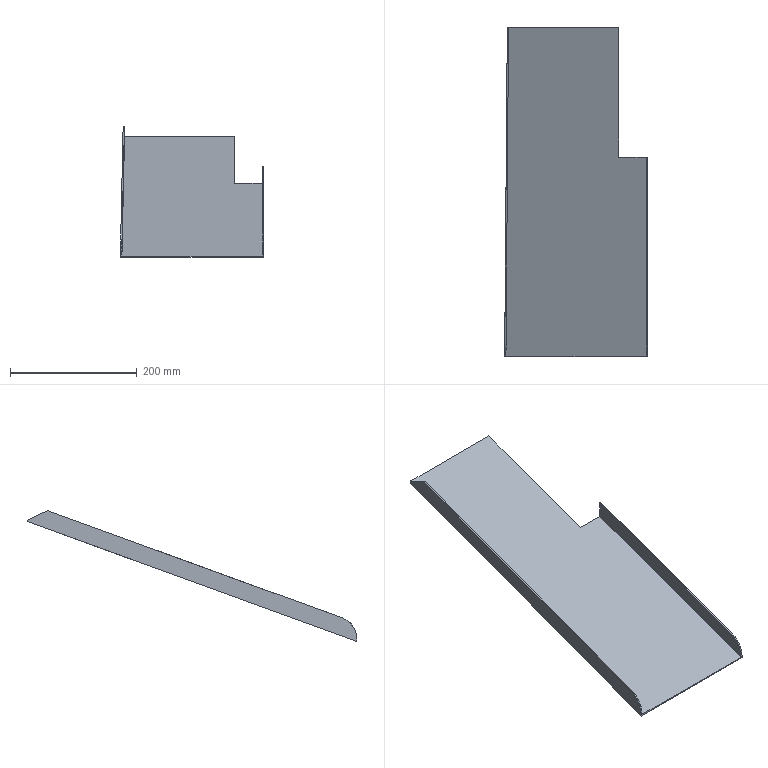Part | NX | features solid 2 | 1 solid | 15 faces | box 225.247 x 520 x 206.353 mm | volume 267602 mm3 | plane 9 | spline 5 | cylinder 1 | commonest cylinder face diameters 70 x1
STEP:
#1=CARTESIAN_POINT('',(-877.991,-100.,-231.58));
#2=VERTEX_POINT('',#1);
#3=CARTESIAN_POINT('',(-882.15,-620.,-420.844));
#4=VERTEX_POINT('',#3);
#5=CARTESIAN_POINT('',(-877.991,-100.,-231.58));
#6=CARTESIAN_POINT('',(-878.46,-143.332,-247.351));
#7=CARTESIAN_POINT('',(-879.198,-229.999,-278.895));
#8=CARTESIAN_POINT('',(-880.069,-338.332,-318.325));
#9=CARTESIAN_POINT('',(-880.798,-424.998,-349.869));
#10=CARTESIAN_POINT('',(-881.335,-511.666,-381.414));
#11=CARTESIAN_POINT('',(-881.837,-576.666,-405.072));
#12=CARTESIAN_POINT('',(-882.15,-620.,-420.844));
#13=B_SPLINE_CURVE_WITH_KNOTS('',3,(#5,#6,#7,#8,#9,#10,#11,#12),.UNSPECIFIED.,.F.,.F.,(4,1,1,1,1,4),(0.8331,0.9714,1.11,1.179,1.248,1.386),.UNSPECIFIED.);
#14=EDGE_CURVE('',#2,#4,#13,.T.);
#15=ORIENTED_EDGE('',*,*,#14,.T.);
#16=CARTESIAN_POINT('',(-660.908,-620.,-420.844));
#17=VERTEX_POINT('',#16);
#18=CARTESIAN_POINT('',(-1178.908,-620.,-420.844));
#19=DIRECTION('',(1.,0.,0.));
#20=VECTOR('',#19,1000.);
#21=LINE('',#18,#20);
#22=EDGE_CURVE('',#4,#17,#21,.T.);
#23=ORIENTED_EDGE('',*,*,#22,.T.);
#24=CARTESIAN_POINT('',(-660.908,-305.,-306.193));
#25=VERTEX_POINT('',#24);
#26=CARTESIAN_POINT('',(-660.908,-100.,-231.58));
#27=DIRECTION('',(0.,-0.9397,-0.342));
#28=VECTOR('',#27,1000.);
#29=LINE('',#26,#28);
#30=EDGE_CURVE('',#25,#17,#29,.T.);
#31=ORIENTED_EDGE('',*,*,#30,.F.);
#32=CARTESIAN_POINT('',(-703.908,-305.,-306.193));
#33=VERTEX_POINT('',#32);
#34=CARTESIAN_POINT('',(-1178.908,-305.,-306.193));
#35=DIRECTION('',(1.,0.,0.));
#36=VECTOR('',#35,1000.);
#37=LINE('',#34,#36);
#38=EDGE_CURVE('',#33,#25,#37,.T.);
#39=ORIENTED_EDGE('',*,*,#38,.F.);
#40=CARTESIAN_POINT('',(-703.908,-100.,-231.58));
#41=VERTEX_POINT('',#40);
#42=CARTESIAN_POINT('',(-703.908,-63.022,-218.121));
#43=DIRECTION('',(0.,-0.9397,-0.342));
#44=VECTOR('',#43,1000.);
#45=LINE('',#42,#44);
#46=EDGE_CURVE('',#41,#33,#45,.T.);
#47=ORIENTED_EDGE('',*,*,#46,.F.);
#48=CARTESIAN_POINT('',(-1178.908,-100.,-231.58));
#49=DIRECTION('',(1.,0.,0.));
#50=VECTOR('',#49,1000.);
#51=LINE('',#48,#50);
#52=EDGE_CURVE('',#2,#41,#51,.T.);
#53=ORIENTED_EDGE('',*,*,#52,.F.);
#54=EDGE_LOOP('',(#15,#23,#31,#39,#47,#53));
#55=FACE_BOUND('',#54,.T.);
#56=CARTESIAN_POINT('',(-1178.908,-63.022,-218.121));
#57=DIRECTION('',(0.,0.342,-0.9397));
#58=DIRECTION('',(-1.,0.,0.));
#59=AXIS2_PLACEMENT_3D('',#56,#57,#58);
#60=PLANE('',#59);
#61=ADVANCED_FACE('',(#55),#60,.F.);
#62=CARTESIAN_POINT('',(-879.998,-100.,-233.708));
#63=VERTEX_POINT('',#62);
#64=CARTESIAN_POINT('',(-703.908,-100.,-233.708));
#65=VERTEX_POINT('',#64);
#66=CARTESIAN_POINT('',(-1178.908,-100.,-233.708));
#67=DIRECTION('',(1.,0.,0.));
#68=VECTOR('',#67,1000.);
#69=LINE('',#66,#68);
#70=EDGE_CURVE('',#63,#65,#69,.T.);
#71=ORIENTED_EDGE('',*,*,#70,.T.);
#72=CARTESIAN_POINT('',(-703.908,-305.,-308.322));
#73=VERTEX_POINT('',#72);
#74=CARTESIAN_POINT('',(-703.908,-62.338,-220.));
#75=DIRECTION('',(0.,-0.9397,-0.342));
#76=VECTOR('',#75,1000.);
#77=LINE('',#74,#76);
#78=EDGE_CURVE('',#65,#73,#77,.T.);
#79=ORIENTED_EDGE('',*,*,#78,.T.);
#80=CARTESIAN_POINT('',(-658.908,-305.,-308.322));
#81=VERTEX_POINT('',#80);
#82=CARTESIAN_POINT('',(-1178.908,-305.,-308.322));
#83=DIRECTION('',(1.,0.,0.));
#84=VECTOR('',#83,1000.);
#85=LINE('',#82,#84);
#86=EDGE_CURVE('',#73,#81,#85,.T.);
#87=ORIENTED_EDGE('',*,*,#86,.T.);
#88=CARTESIAN_POINT('',(-658.908,-620.,-422.972));
#89=VERTEX_POINT('',#88);
#90=CARTESIAN_POINT('',(-658.908,-62.338,-220.));
#91=DIRECTION('',(0.,-0.9397,-0.342));
#92=VECTOR('',#91,1000.);
#93=LINE('',#90,#92);
#94=EDGE_CURVE('',#81,#89,#93,.T.);
#95=ORIENTED_EDGE('',*,*,#94,.T.);
#96=CARTESIAN_POINT('',(-884.155,-620.,-422.972));
#97=VERTEX_POINT('',#96);
#98=CARTESIAN_POINT('',(-1178.908,-620.,-422.972));
#99=DIRECTION('',(1.,0.,0.));
#100=VECTOR('',#99,1000.);
#101=LINE('',#98,#100);
#102=EDGE_CURVE('',#97,#89,#101,.T.);
#103=ORIENTED_EDGE('',*,*,#102,.F.);
#104=CARTESIAN_POINT('',(-879.998,-100.,-233.708));
#105=CARTESIAN_POINT('',(-880.468,-143.332,-249.48));
#106=CARTESIAN_POINT('',(-881.204,-229.999,-281.024));
#107=CARTESIAN_POINT('',(-882.073,-338.332,-320.454));
#108=CARTESIAN_POINT('',(-882.805,-424.999,-351.998));
#109=CARTESIAN_POINT('',(-883.339,-511.666,-383.542));
#110=CARTESIAN_POINT('',(-883.842,-576.666,-407.2));
#111=CARTESIAN_POINT('',(-884.155,-620.,-422.972));
#112=B_SPLINE_CURVE_WITH_KNOTS('',3,(#104,#105,#106,#107,#108,#109,#110,#111),.UNSPECIFIED.,.F.,.F.,(4,1,1,1,1,4),(2.341,2.479,2.617,2.687,2.756,2.894),.UNSPECIFIED.);
#113=EDGE_CURVE('',#63,#97,#112,.T.);
#114=ORIENTED_EDGE('',*,*,#113,.F.);
#115=EDGE_LOOP('',(#71,#79,#87,#95,#103,#114));
#116=FACE_BOUND('',#115,.T.);
#117=CARTESIAN_POINT('',(-1178.908,-62.338,-220.));
#118=DIRECTION('',(0.,0.342,-0.9397));
#119=DIRECTION('',(-1.,0.,0.));
#120=AXIS2_PLACEMENT_3D('',#117,#118,#119);
#121=PLANE('',#120);
#122=ADVANCED_FACE('',(#116),#121,.T.);
#123=CARTESIAN_POINT('',(-877.991,-100.,-231.556));
#124=VERTEX_POINT('',#123);
#125=CARTESIAN_POINT('',(-878.237,-132.013,-216.627));
#126=VERTEX_POINT('',#125);
#127=CARTESIAN_POINT('',(-877.991,-100.,-231.556));
#128=CARTESIAN_POINT('',(-878.076,-110.671,-226.579));
#129=CARTESIAN_POINT('',(-878.158,-121.342,-221.603));
#130=CARTESIAN_POINT('',(-878.237,-132.013,-216.627));
#131=B_SPLINE_CURVE_WITH_KNOTS('',3,(#127,#128,#129,#130),.UNSPECIFIED.,.F.,.F.,(4,4),(0.00003167,0.03536),.UNSPECIFIED.);
#132=EDGE_CURVE('',#124,#126,#131,.T.);
#133=ORIENTED_EDGE('',*,*,#132,.F.);
#134=CARTESIAN_POINT('',(-879.991,-100.,-231.54));
#135=VERTEX_POINT('',#134);
#136=CARTESIAN_POINT('',(-877.991,-100.,-231.556));
#137=CARTESIAN_POINT('',(-878.658,-100.,-231.55));
#138=CARTESIAN_POINT('',(-879.324,-100.,-231.545));
#139=CARTESIAN_POINT('',(-879.991,-100.,-231.54));
#140=B_SPLINE_CURVE_WITH_KNOTS('',3,(#136,#137,#138,#139),.UNSPECIFIED.,.F.,.F.,(4,4),(0.003,0.005),.UNSPECIFIED.);
#141=EDGE_CURVE('',#124,#135,#140,.T.);
#142=ORIENTED_EDGE('',*,*,#141,.T.);
#143=CARTESIAN_POINT('',(-880.237,-131.994,-216.62));
#144=VERTEX_POINT('',#143);
#145=CARTESIAN_POINT('',(-880.237,-131.994,-216.62));
#146=CARTESIAN_POINT('',(-880.158,-121.329,-221.593));
#147=CARTESIAN_POINT('',(-880.076,-110.665,-226.566));
#148=CARTESIAN_POINT('',(-879.991,-100.,-231.54));
#149=B_SPLINE_CURVE_WITH_KNOTS('',3,(#145,#146,#147,#148),.UNSPECIFIED.,.F.,.F.,(4,4),(0.,0.0353),.UNSPECIFIED.);
#150=EDGE_CURVE('',#144,#135,#149,.T.);
#151=ORIENTED_EDGE('',*,*,#150,.F.);
#152=CARTESIAN_POINT('',(-878.237,-132.013,-216.627));
#153=CARTESIAN_POINT('',(-878.904,-132.007,-216.625));
#154=CARTESIAN_POINT('',(-879.571,-132.,-216.622));
#155=CARTESIAN_POINT('',(-880.237,-131.994,-216.62));
#156=B_SPLINE_CURVE_WITH_KNOTS('',3,(#152,#153,#154,#155),.UNSPECIFIED.,.F.,.F.,(4,4),(0.005001,0.007001),.UNSPECIFIED.);
#157=EDGE_CURVE('',#126,#144,#156,.T.);
#158=ORIENTED_EDGE('',*,*,#157,.F.);
#159=EDGE_LOOP('',(#133,#142,#151,#158));
#160=FACE_BOUND('',#159,.T.);
#161=CARTESIAN_POINT('',(-878.225,-132.013,-216.627));
#162=CARTESIAN_POINT('',(-878.896,-132.007,-216.625));
#163=CARTESIAN_POINT('',(-879.567,-132.,-216.622));
#164=CARTESIAN_POINT('',(-880.237,-131.994,-216.62));
#165=CARTESIAN_POINT('',(-880.244,-131.994,-216.62));
#166=CARTESIAN_POINT('',(-880.25,-131.994,-216.62));
#167=CARTESIAN_POINT('',(-880.257,-131.994,-216.62));
#168=CARTESIAN_POINT('',(-877.971,-99.971,-231.569));
#169=CARTESIAN_POINT('',(-878.641,-99.965,-231.567));
#170=CARTESIAN_POINT('',(-879.312,-99.959,-231.564));
#171=CARTESIAN_POINT('',(-879.983,-99.952,-231.562));
#172=CARTESIAN_POINT('',(-879.989,-99.952,-231.562));
#173=CARTESIAN_POINT('',(-879.996,-99.952,-231.562));
#174=CARTESIAN_POINT('',(-880.003,-99.952,-231.562));
#175=CARTESIAN_POINT('',(-877.969,-99.808,-231.645));
#176=CARTESIAN_POINT('',(-878.64,-99.802,-231.643));
#177=CARTESIAN_POINT('',(-879.311,-99.795,-231.641));
#178=CARTESIAN_POINT('',(-879.981,-99.789,-231.638));
#179=CARTESIAN_POINT('',(-879.988,-99.789,-231.638));
#180=CARTESIAN_POINT('',(-879.995,-99.789,-231.638));
#181=CARTESIAN_POINT('',(-880.001,-99.789,-231.638));
#182=B_SPLINE_SURFACE_WITH_KNOTS('',1,3,((#161,#162,#163,#164,#165,#166,#167),(#168,#169,#170,#171,#172,#173,#174),(#175,#176,#177,#178,#179,#180,#181)),.PLANE_SURF.,.F.,.F.,.F.,(2,1,2),(4,3,4),(0.,1.,1.005),(0.01298,0.01499,0.01501),.PIECEWISE_BEZIER_KNOTS.);
#183=ADVANCED_FACE('',(#160),#182,.T.);
#184=CARTESIAN_POINT('',(-877.991,-100.,-231.58));
#185=CARTESIAN_POINT('',(-877.991,-100.,-231.572));
#186=CARTESIAN_POINT('',(-877.991,-100.,-231.564));
#187=CARTESIAN_POINT('',(-877.991,-100.,-231.556));
#188=B_SPLINE_CURVE_WITH_KNOTS('',3,(#184,#185,#186,#187),.UNSPECIFIED.,.F.,.F.,(4,4),(0.002931,0.002955),.UNSPECIFIED.);
#189=EDGE_CURVE('',#2,#124,#188,.T.);
#190=ORIENTED_EDGE('',*,*,#189,.F.);
#191=ORIENTED_EDGE('',*,*,#52,.T.);
#192=CARTESIAN_POINT('',(-703.908,-100.,0.000000017));
#193=DIRECTION('',(0.,0.,-1.));
#194=VECTOR('',#193,1000.);
#195=LINE('',#192,#194);
#196=EDGE_CURVE('',#41,#65,#195,.T.);
#197=ORIENTED_EDGE('',*,*,#196,.T.);
#198=ORIENTED_EDGE('',*,*,#70,.F.);
#199=CARTESIAN_POINT('',(-879.991,-100.,-231.54));
#200=CARTESIAN_POINT('',(-879.993,-100.,-232.262));
#201=CARTESIAN_POINT('',(-879.996,-100.,-232.985));
#202=CARTESIAN_POINT('',(-879.998,-100.,-233.708));
#203=B_SPLINE_CURVE_WITH_KNOTS('',3,(#199,#200,#201,#202),.UNSPECIFIED.,.F.,.F.,(4,4),(0.06045,0.06262),.UNSPECIFIED.);
#204=EDGE_CURVE('',#135,#63,#203,.T.);
#205=ORIENTED_EDGE('',*,*,#204,.F.);
#206=ORIENTED_EDGE('',*,*,#141,.F.);
#207=EDGE_LOOP('',(#190,#191,#197,#198,#205,#206));
#208=FACE_BOUND('',#207,.T.);
#209=CARTESIAN_POINT('',(2851.092,-100.,0.000000017));
#210=DIRECTION('',(0.,1.,0.));
#211=DIRECTION('',(0.,0.,1.));
#212=AXIS2_PLACEMENT_3D('',#209,#210,#211);
#213=PLANE('',#212);
#214=ADVANCED_FACE('',(#208),#213,.T.);
#215=ORIENTED_EDGE('',*,*,#196,.F.);
#216=ORIENTED_EDGE('',*,*,#46,.T.);
#217=CARTESIAN_POINT('',(-703.908,-305.,-570.));
#218=DIRECTION('',(0.,0.,-1.));
#219=VECTOR('',#218,1000.);
#220=LINE('',#217,#219);
#221=EDGE_CURVE('',#33,#73,#220,.T.);
#222=ORIENTED_EDGE('',*,*,#221,.T.);
#223=ORIENTED_EDGE('',*,*,#78,.F.);
#224=EDGE_LOOP('',(#215,#216,#222,#223));
#225=FACE_BOUND('',#224,.T.);
#226=CARTESIAN_POINT('',(-703.908,574.883,14.058));
#227=DIRECTION('',(1.,0.,0.));
#228=DIRECTION('',(0.,0.,-1.));
#229=AXIS2_PLACEMENT_3D('',#226,#227,#228);
#230=PLANE('',#229);
#231=ADVANCED_FACE('',(#225),#230,.T.);
#232=ORIENTED_EDGE('',*,*,#113,.T.);
#233=CARTESIAN_POINT('',(-884.145,-620.,-418.747));
#234=VERTEX_POINT('',#233);
#235=CARTESIAN_POINT('',(-884.145,-620.,-418.747));
#236=CARTESIAN_POINT('',(-884.148,-620.,-420.155));
#237=CARTESIAN_POINT('',(-884.152,-620.,-421.564));
#238=CARTESIAN_POINT('',(-884.155,-620.,-422.972));
#239=B_SPLINE_CURVE_WITH_KNOTS('',3,(#235,#236,#237,#238),.UNSPECIFIED.,.F.,.F.,(4,4),(0.06426,0.06848),.UNSPECIFIED.);
#240=EDGE_CURVE('',#234,#97,#239,.T.);
#241=ORIENTED_EDGE('',*,*,#240,.F.);
#242=CARTESIAN_POINT('',(-883.922,-596.971,-385.858));
#243=VERTEX_POINT('',#242);
#244=CARTESIAN_POINT('',(-883.922,-596.971,-385.858));
#245=CARTESIAN_POINT('',(-883.946,-600.306,-387.072));
#246=CARTESIAN_POINT('',(-883.995,-606.652,-390.551));
#247=CARTESIAN_POINT('',(-884.06,-614.122,-398.358));
#248=CARTESIAN_POINT('',(-884.113,-618.905,-408.081));
#249=CARTESIAN_POINT('',(-884.137,-620.,-415.15));
#250=CARTESIAN_POINT('',(-884.145,-620.,-418.747));
#251=B_SPLINE_CURVE_WITH_KNOTS('',3,(#244,#245,#246,#247,#248,#249,#250),.UNSPECIFIED.,.F.,.F.,(4,1,1,1,4),(0.01625,0.0269,0.03754,0.04818,0.05882),.UNSPECIFIED.);
#252=EDGE_CURVE('',#234,#243,#251,.F.);
#253=ORIENTED_EDGE('',*,*,#252,.T.);
#254=CARTESIAN_POINT('',(-880.237,-131.994,-216.62));
#255=CARTESIAN_POINT('',(-880.63,-170.741,-230.723));
#256=CARTESIAN_POINT('',(-881.267,-248.237,-258.929));
#257=CARTESIAN_POINT('',(-882.569,-403.229,-315.341));
#258=CARTESIAN_POINT('',(-883.363,-519.474,-357.651));
#259=CARTESIAN_POINT('',(-883.922,-596.971,-385.858));
#260=B_SPLINE_CURVE_WITH_KNOTS('',3,(#254,#255,#256,#257,#258,#259),.UNSPECIFIED.,.F.,.F.,(4,1,1,4),(2.365,2.489,2.612,2.86),.UNSPECIFIED.);
#261=EDGE_CURVE('',#144,#243,#260,.T.);
#262=ORIENTED_EDGE('',*,*,#261,.F.);
#263=ORIENTED_EDGE('',*,*,#150,.T.);
#264=ORIENTED_EDGE('',*,*,#204,.T.);
#265=EDGE_LOOP('',(#232,#241,#253,#262,#263,#264));
#266=FACE_BOUND('',#265,.T.);
#267=CARTESIAN_POINT('',(-879.956,-105.275,-206.895));
#268=CARTESIAN_POINT('',(-879.956,-96.041,-232.267));
#269=CARTESIAN_POINT('',(-880.018,-111.007,-208.981));
#270=CARTESIAN_POINT('',(-880.018,-101.773,-234.353));
#271=CARTESIAN_POINT('',(-880.141,-122.433,-213.14));
#272=CARTESIAN_POINT('',(-880.141,-113.198,-238.512));
#273=CARTESIAN_POINT('',(-880.31,-139.15,-219.225));
#274=CARTESIAN_POINT('',(-880.31,-129.915,-244.596));
#275=CARTESIAN_POINT('',(-880.442,-152.781,-224.186));
#276=CARTESIAN_POINT('',(-880.442,-143.546,-249.557));
#277=CARTESIAN_POINT('',(-880.54,-163.506,-228.089));
#278=CARTESIAN_POINT('',(-880.54,-154.272,-253.461));
#279=CARTESIAN_POINT('',(-880.599,-170.114,-230.494));
#280=CARTESIAN_POINT('',(-880.599,-160.879,-255.866));
#281=CARTESIAN_POINT('',(-880.645,-175.397,-232.417));
#282=CARTESIAN_POINT('',(-880.645,-166.163,-257.789));
#283=CARTESIAN_POINT('',(-880.693,-180.936,-234.433));
#284=CARTESIAN_POINT('',(-880.693,-171.702,-259.805));
#285=CARTESIAN_POINT('',(-880.752,-187.772,-236.922));
#286=CARTESIAN_POINT('',(-880.752,-178.538,-262.293));
#287=CARTESIAN_POINT('',(-880.823,-196.013,-239.921));
#288=CARTESIAN_POINT('',(-880.823,-186.778,-265.293));
#289=CARTESIAN_POINT('',(-880.894,-204.244,-242.917));
#290=CARTESIAN_POINT('',(-880.894,-195.009,-268.288));
#291=CARTESIAN_POINT('',(-880.965,-212.477,-245.913));
#292=CARTESIAN_POINT('',(-880.965,-203.243,-271.285));
#293=CARTESIAN_POINT('',(-881.023,-219.338,-248.41));
#294=CARTESIAN_POINT('',(-881.023,-210.103,-273.782));
#295=CARTESIAN_POINT('',(-881.07,-224.826,-250.408));
#296=CARTESIAN_POINT('',(-881.07,-215.592,-275.78));
#297=CARTESIAN_POINT('',(-881.106,-228.942,-251.906));
#298=CARTESIAN_POINT('',(-881.106,-219.708,-277.278));
#299=CARTESIAN_POINT('',(-881.135,-232.374,-253.155));
#300=CARTESIAN_POINT('',(-881.135,-223.139,-278.527));
#301=CARTESIAN_POINT('',(-881.159,-235.116,-254.153));
#302=CARTESIAN_POINT('',(-881.159,-225.882,-279.525));
#303=CARTESIAN_POINT('',(-881.173,-236.836,-254.779));
#304=CARTESIAN_POINT('',(-881.173,-227.601,-280.151));
#305=CARTESIAN_POINT('',(-881.184,-238.029,-255.213));
#306=CARTESIAN_POINT('',(-881.184,-228.794,-280.585));
#307=CARTESIAN_POINT('',(-881.189,-238.727,-255.468));
#308=CARTESIAN_POINT('',(-881.189,-229.492,-280.839));
#309=CARTESIAN_POINT('',(-881.194,-239.204,-255.641));
#310=CARTESIAN_POINT('',(-881.194,-229.969,-281.013));
#311=CARTESIAN_POINT('',(-881.2,-239.931,-255.906));
#312=CARTESIAN_POINT('',(-881.2,-230.696,-281.277));
#313=CARTESIAN_POINT('',(-881.207,-240.811,-256.226));
#314=CARTESIAN_POINT('',(-881.207,-231.576,-281.598));
#315=CARTESIAN_POINT('',(-881.221,-242.387,-256.8));
#316=CARTESIAN_POINT('',(-881.221,-233.153,-282.172));
#317=CARTESIAN_POINT('',(-881.24,-244.606,-257.607));
#318=CARTESIAN_POINT('',(-881.24,-235.371,-282.979));
#319=CARTESIAN_POINT('',(-881.27,-248.139,-258.893));
#320=CARTESIAN_POINT('',(-881.27,-238.905,-284.265));
#321=CARTESIAN_POINT('',(-881.307,-252.501,-260.481));
#322=CARTESIAN_POINT('',(-881.307,-243.267,-285.853));
#323=CARTESIAN_POINT('',(-881.365,-259.375,-262.983));
#324=CARTESIAN_POINT('',(-881.365,-250.14,-288.355));
#325=CARTESIAN_POINT('',(-881.436,-267.763,-266.036));
#326=CARTESIAN_POINT('',(-881.436,-258.529,-291.408));
#327=CARTESIAN_POINT('',(-881.546,-280.751,-270.763));
#328=CARTESIAN_POINT('',(-881.546,-271.517,-296.135));
#329=CARTESIAN_POINT('',(-881.675,-296.174,-276.377));
#330=CARTESIAN_POINT('',(-881.675,-286.939,-301.748));
#331=CARTESIAN_POINT('',(-881.817,-313.381,-282.64));
#332=CARTESIAN_POINT('',(-881.817,-304.147,-308.011));
#333=CARTESIAN_POINT('',(-881.925,-326.638,-287.464));
#334=CARTESIAN_POINT('',(-881.925,-317.403,-312.836));
#335=CARTESIAN_POINT('',(-882.005,-336.593,-291.088));
#336=CARTESIAN_POINT('',(-882.005,-327.358,-316.46));
#337=CARTESIAN_POINT('',(-882.062,-343.734,-293.687));
#338=CARTESIAN_POINT('',(-882.062,-334.5,-319.059));
#339=CARTESIAN_POINT('',(-882.116,-350.551,-296.168));
#340=CARTESIAN_POINT('',(-882.116,-341.316,-321.54));
#341=CARTESIAN_POINT('',(-882.158,-355.961,-298.137));
#342=CARTESIAN_POINT('',(-882.158,-346.726,-323.509));
#343=CARTESIAN_POINT('',(-882.19,-360.126,-299.653));
#344=CARTESIAN_POINT('',(-882.19,-350.891,-325.025));
#345=CARTESIAN_POINT('',(-882.209,-362.662,-300.576));
#346=CARTESIAN_POINT('',(-882.209,-353.427,-325.948));
#347=CARTESIAN_POINT('',(-882.224,-364.649,-301.299));
#348=CARTESIAN_POINT('',(-882.224,-355.414,-326.671));
#349=CARTESIAN_POINT('',(-882.236,-366.122,-301.835));
#350=CARTESIAN_POINT('',(-882.236,-356.887,-327.207));
#351=CARTESIAN_POINT('',(-882.245,-367.323,-302.273));
#352=CARTESIAN_POINT('',(-882.245,-358.089,-327.645));
#353=CARTESIAN_POINT('',(-882.252,-368.294,-302.626));
#354=CARTESIAN_POINT('',(-882.252,-359.06,-327.998));
#355=CARTESIAN_POINT('',(-882.256,-368.852,-302.829));
#356=CARTESIAN_POINT('',(-882.256,-359.618,-328.201));
#357=CARTESIAN_POINT('',(-882.26,-369.398,-303.028));
#358=CARTESIAN_POINT('',(-882.26,-360.163,-328.4));
#359=CARTESIAN_POINT('',(-882.266,-370.118,-303.29));
#360=CARTESIAN_POINT('',(-882.266,-360.884,-328.662));
#361=CARTESIAN_POINT('',(-882.275,-371.298,-303.719));
#362=CARTESIAN_POINT('',(-882.275,-362.063,-329.091));
#363=CARTESIAN_POINT('',(-882.293,-373.714,-304.599));
#364=CARTESIAN_POINT('',(-882.293,-364.479,-329.97));
#365=CARTESIAN_POINT('',(-882.319,-377.135,-305.844));
#366=CARTESIAN_POINT('',(-882.319,-367.901,-331.216));
#367=CARTESIAN_POINT('',(-882.351,-381.254,-307.343));
#368=CARTESIAN_POINT('',(-882.351,-372.02,-332.715));
#369=CARTESIAN_POINT('',(-882.393,-386.742,-309.34));
#370=CARTESIAN_POINT('',(-882.393,-377.507,-334.712));
#371=CARTESIAN_POINT('',(-882.447,-393.602,-311.838));
#372=CARTESIAN_POINT('',(-882.447,-384.368,-337.209));
#373=CARTESIAN_POINT('',(-882.512,-401.834,-314.834));
#374=CARTESIAN_POINT('',(-882.512,-392.6,-340.206));
#375=CARTESIAN_POINT('',(-882.579,-410.067,-317.83));
#376=CARTESIAN_POINT('',(-882.579,-400.832,-343.202));
#377=CARTESIAN_POINT('',(-882.646,-418.299,-320.826));
#378=CARTESIAN_POINT('',(-882.646,-409.064,-346.198));
#379=CARTESIAN_POINT('',(-882.703,-425.159,-323.323));
#380=CARTESIAN_POINT('',(-882.703,-415.925,-348.695));
#381=CARTESIAN_POINT('',(-882.75,-430.647,-325.321));
#382=CARTESIAN_POINT('',(-882.75,-421.413,-350.693));
#383=CARTESIAN_POINT('',(-882.779,-434.077,-326.569));
#384=CARTESIAN_POINT('',(-882.779,-424.843,-351.941));
#385=CARTESIAN_POINT('',(-882.802,-436.822,-327.568));
#386=CARTESIAN_POINT('',(-882.802,-427.587,-352.94));
#387=CARTESIAN_POINT('',(-882.817,-438.537,-328.192));
#388=CARTESIAN_POINT('',(-882.817,-429.302,-353.564));
#389=CARTESIAN_POINT('',(-882.829,-439.909,-328.692));
#390=CARTESIAN_POINT('',(-882.829,-430.674,-354.063));
#391=CARTESIAN_POINT('',(-882.838,-440.937,-329.066));
#392=CARTESIAN_POINT('',(-882.838,-431.703,-354.438));
#393=CARTESIAN_POINT('',(-882.845,-441.796,-329.379));
#394=CARTESIAN_POINT('',(-882.845,-432.562,-354.75));
#395=CARTESIAN_POINT('',(-882.851,-442.48,-329.627));
#396=CARTESIAN_POINT('',(-882.851,-433.245,-354.999));
#397=CARTESIAN_POINT('',(-882.855,-442.915,-329.786));
#398=CARTESIAN_POINT('',(-882.855,-433.68,-355.157));
#399=CARTESIAN_POINT('',(-882.857,-443.245,-329.906));
#400=CARTESIAN_POINT('',(-882.857,-434.01,-355.278));
#401=CARTESIAN_POINT('',(-882.86,-443.541,-330.014));
#402=CARTESIAN_POINT('',(-882.86,-434.306,-355.385));
#403=CARTESIAN_POINT('',(-882.86,-443.499,-329.998));
#404=CARTESIAN_POINT('',(-882.86,-434.264,-355.37));
#405=CARTESIAN_POINT('',(-882.86,-443.573,-330.025));
#406=CARTESIAN_POINT('',(-882.86,-434.338,-355.397));
#407=CARTESIAN_POINT('',(-882.86,-443.656,-330.056));
#408=CARTESIAN_POINT('',(-882.86,-434.422,-355.427));
#409=CARTESIAN_POINT('',(-882.862,-443.996,-330.179));
#410=CARTESIAN_POINT('',(-882.862,-434.761,-355.551));
#411=CARTESIAN_POINT('',(-882.866,-444.894,-330.506));
#412=CARTESIAN_POINT('',(-882.866,-435.659,-355.878));
#413=CARTESIAN_POINT('',(-882.875,-446.96,-331.258));
#414=CARTESIAN_POINT('',(-882.875,-437.726,-356.63));
#415=CARTESIAN_POINT('',(-882.885,-449.161,-332.059));
#416=CARTESIAN_POINT('',(-882.885,-439.926,-357.431));
#417=CARTESIAN_POINT('',(-882.892,-450.89,-332.688));
#418=CARTESIAN_POINT('',(-882.892,-441.655,-358.06));
#419=CARTESIAN_POINT('',(-882.895,-451.667,-332.971));
#420=CARTESIAN_POINT('',(-882.895,-442.433,-358.343));
#421=CARTESIAN_POINT('',(-882.898,-452.288,-333.197));
#422=CARTESIAN_POINT('',(-882.898,-443.053,-358.569));
#423=CARTESIAN_POINT('',(-882.9,-452.845,-333.4));
#424=CARTESIAN_POINT('',(-882.9,-443.61,-358.772));
#425=CARTESIAN_POINT('',(-882.901,-453.091,-333.49));
#426=CARTESIAN_POINT('',(-882.901,-443.857,-358.861));
#427=CARTESIAN_POINT('',(-882.903,-453.523,-333.647));
#428=CARTESIAN_POINT('',(-882.903,-444.288,-359.019));
#429=CARTESIAN_POINT('',(-882.905,-454.018,-333.827));
#430=CARTESIAN_POINT('',(-882.905,-444.783,-359.199));
#431=CARTESIAN_POINT('',(-882.909,-454.814,-334.117));
#432=CARTESIAN_POINT('',(-882.909,-445.58,-359.489));
#433=CARTESIAN_POINT('',(-882.915,-456.155,-334.605));
#434=CARTESIAN_POINT('',(-882.915,-446.921,-359.977));
#435=CARTESIAN_POINT('',(-882.924,-457.951,-335.259));
#436=CARTESIAN_POINT('',(-882.924,-448.717,-360.63));
#437=CARTESIAN_POINT('',(-882.933,-459.587,-335.854));
#438=CARTESIAN_POINT('',(-882.933,-450.352,-361.226));
#439=CARTESIAN_POINT('',(-882.941,-460.784,-336.29));
#440=CARTESIAN_POINT('',(-882.941,-451.55,-361.661));
#441=CARTESIAN_POINT('',(-882.945,-461.447,-336.531));
#442=CARTESIAN_POINT('',(-882.945,-452.213,-361.903));
#443=CARTESIAN_POINT('',(-882.947,-461.831,-336.671));
#444=CARTESIAN_POINT('',(-882.947,-452.597,-362.043));
#445=CARTESIAN_POINT('',(-882.949,-462.096,-336.767));
#446=CARTESIAN_POINT('',(-882.949,-452.862,-362.139));
#447=CARTESIAN_POINT('',(-882.949,-462.063,-336.755));
#448=CARTESIAN_POINT('',(-882.949,-452.828,-362.127));
#449=CARTESIAN_POINT('',(-882.949,-462.107,-336.771));
#450=CARTESIAN_POINT('',(-882.949,-452.872,-362.143));
#451=CARTESIAN_POINT('',(-882.95,-462.152,-336.788));
#452=CARTESIAN_POINT('',(-882.95,-452.918,-362.159));
#453=CARTESIAN_POINT('',(-882.951,-462.338,-336.855));
#454=CARTESIAN_POINT('',(-882.951,-453.103,-362.227));
#455=CARTESIAN_POINT('',(-882.954,-462.811,-337.027));
#456=CARTESIAN_POINT('',(-882.954,-453.576,-362.399));
#457=CARTESIAN_POINT('',(-882.962,-463.882,-337.417));
#458=CARTESIAN_POINT('',(-882.962,-454.648,-362.789));
#459=CARTESIAN_POINT('',(-882.973,-465.387,-337.965));
#460=CARTESIAN_POINT('',(-882.973,-456.153,-363.337));
#461=CARTESIAN_POINT('',(-882.987,-467.328,-338.671));
#462=CARTESIAN_POINT('',(-882.987,-458.093,-364.043));
#463=CARTESIAN_POINT('',(-883.004,-469.704,-339.536));
#464=CARTESIAN_POINT('',(-883.004,-460.469,-364.908));
#465=CARTESIAN_POINT('',(-883.021,-472.046,-340.389));
#466=CARTESIAN_POINT('',(-883.021,-462.811,-365.76));
#467=CARTESIAN_POINT('',(-883.036,-474.138,-341.15));
#468=CARTESIAN_POINT('',(-883.036,-464.903,-366.522));
#469=CARTESIAN_POINT('',(-883.048,-475.815,-341.76));
#470=CARTESIAN_POINT('',(-883.048,-466.58,-367.132));
#471=CARTESIAN_POINT('',(-883.059,-477.304,-342.303));
#472=CARTESIAN_POINT('',(-883.059,-468.07,-367.674));
#473=CARTESIAN_POINT('',(-883.068,-478.547,-342.755));
#474=CARTESIAN_POINT('',(-883.068,-469.312,-368.127));
#475=CARTESIAN_POINT('',(-883.074,-479.355,-343.049));
#476=CARTESIAN_POINT('',(-883.074,-470.12,-368.421));
#477=CARTESIAN_POINT('',(-883.078,-479.995,-343.282));
#478=CARTESIAN_POINT('',(-883.078,-470.76,-368.654));
#479=CARTESIAN_POINT('',(-883.081,-480.445,-343.446));
#480=CARTESIAN_POINT('',(-883.081,-471.21,-368.817));
#481=CARTESIAN_POINT('',(-883.083,-480.708,-343.541));
#482=CARTESIAN_POINT('',(-883.083,-471.473,-368.913));
#483=CARTESIAN_POINT('',(-883.084,-480.857,-343.596));
#484=CARTESIAN_POINT('',(-883.084,-471.622,-368.967));
#485=CARTESIAN_POINT('',(-883.087,-481.171,-343.71));
#486=CARTESIAN_POINT('',(-883.087,-471.936,-369.082));
#487=CARTESIAN_POINT('',(-883.09,-481.592,-343.863));
#488=CARTESIAN_POINT('',(-883.09,-472.358,-369.235));
#489=CARTESIAN_POINT('',(-883.095,-482.281,-344.114));
#490=CARTESIAN_POINT('',(-883.095,-473.047,-369.486));
#491=CARTESIAN_POINT('',(-883.101,-483.137,-344.426));
#492=CARTESIAN_POINT('',(-883.101,-473.903,-369.797));
#493=CARTESIAN_POINT('',(-883.116,-485.196,-345.175));
#494=CARTESIAN_POINT('',(-883.116,-475.962,-370.547));
#495=CARTESIAN_POINT('',(-883.138,-488.283,-346.299));
#496=CARTESIAN_POINT('',(-883.138,-479.049,-371.67));
#497=CARTESIAN_POINT('',(-883.168,-492.4,-347.797));
#498=CARTESIAN_POINT('',(-883.168,-483.166,-373.169));
#499=CARTESIAN_POINT('',(-883.197,-496.517,-349.295));
#500=CARTESIAN_POINT('',(-883.197,-487.282,-374.667));
#501=CARTESIAN_POINT('',(-883.237,-502.005,-351.293));
#502=CARTESIAN_POINT('',(-883.237,-492.771,-376.665));
#503=CARTESIAN_POINT('',(-883.286,-508.866,-353.79));
#504=CARTESIAN_POINT('',(-883.286,-499.631,-379.162));
#505=CARTESIAN_POINT('',(-883.366,-519.842,-357.785));
#506=CARTESIAN_POINT('',(-883.366,-510.608,-383.157));
#507=CARTESIAN_POINT('',(-883.465,-533.564,-362.78));
#508=CARTESIAN_POINT('',(-883.465,-524.33,-388.151));
#509=CARTESIAN_POINT('',(-883.583,-550.03,-368.773));
#510=CARTESIAN_POINT('',(-883.583,-540.796,-394.144));
#511=CARTESIAN_POINT('',(-883.742,-571.985,-376.763));
#512=CARTESIAN_POINT('',(-883.742,-562.75,-402.135));
#513=CARTESIAN_POINT('',(-883.94,-599.427,-386.752));
#514=CARTESIAN_POINT('',(-883.94,-590.193,-412.124));
#515=CARTESIAN_POINT('',(-884.098,-621.381,-394.742));
#516=CARTESIAN_POINT('',(-884.098,-612.147,-420.114));
#517=CARTESIAN_POINT('',(-884.177,-632.358,-398.738));
#518=CARTESIAN_POINT('',(-884.177,-623.124,-424.109));
#519=B_SPLINE_SURFACE_WITH_KNOTS('',3,1,((#267,#268),(#269,#270),(#271,#272),(#273,#274),(#275,#276),(#277,#278),(#279,#280),(#281,#282),(#283,#284),(#285,#286),(#287,#288),(#289,#290),(#291,#292),(#293,#294),(#295,#296),(#297,#298),(#299,#300),(#301,#302),(#303,#304),(#305,#306),(#307,#308),(#309,#310),(#311,#312),(#313,#314),(#315,#316),(#317,#318),(#319,#320),(#321,#322),(#323,#324),(#325,#326),(#327,#328),(#329,#330),(#331,#332),(#333,#334),(#335,#336),(#337,#338),(#339,#340),(#341,#342),(#343,#344),(#345,#346),(#347,#348),(#349,#350),(#351,#352),(#353,#354),(#355,#356),(#357,#358),(#359,#360),(#361,#362),(#363,#364),(#365,#366),(#367,#368),(#369,#370),(#371,#372),(#373,#374),(#375,#376),(#377,#378),(#379,#380),(#381,#382),(#383,#384),(#385,#386),(#387,#388),(#389,#390),(#391,#392),(#393,#394),(#395,#396),(#397,#398),(#399,#400),(#401,#402),(#403,#404),(#405,#406),(#407,#408),(#409,#410),(#411,#412),(#413,#414),(#415,#416),(#417,#418),(#419,#420),(#421,#422),(#423,#424),(#425,#426),(#427,#428),(#429,#430),(#431,#432),(#433,#434),(#435,#436),(#437,#438),(#439,#440),(#441,#442),(#443,#444),(#445,#446),(#447,#448),(#449,#450),(#451,#452),(#453,#454),(#455,#456),(#457,#458),(#459,#460),(#461,#462),(#463,#464),(#465,#466),(#467,#468),(#469,#470),(#471,#472),(#473,#474),(#475,#476),(#477,#478),(#479,#480),(#481,#482),(#483,#484),(#485,#486),(#487,#488),(#489,#490),(#491,#492),(#493,#494),(#495,#496),(#497,#498),(#499,#500),(#501,#502),(#503,#504),(#505,#506),(#507,#508),(#509,#510),(#511,#512),(#513,#514),(#515,#516),(#517,#518)),.SURF_OF_LINEAR_EXTRUSION.,.F.,.F.,.F.,(4,1,1,1,1,1,1,1,1,1,1,1,1,1,1,1,1,1,1,1,1,1,1,1,1,1,1,1,1,1,1,1,1,1,1,1,1,1,1,1,1,1,1,1,1,1,1,1,1,1,1,1,1,1,1,1,1,1,1,1,1,1,1,1,1,1,1,1,1,1,1,1,1,1,1,1,1,1,1,1,1,1,1,1,1,1,1,1,1,1,1,1,1,1,1,1,1,1,1,1,1,1,1,1,1,1,1,1,1,1,1,1,1,1,1,1,1,1,1,1,1,1,1,4),(2,2),(-0.007203,0.02446,0.05613,0.08779,0.1036,0.1195,0.1274,0.1353,0.1511,0.167,0.1828,0.1986,0.2145,0.2224,0.2303,0.2382,0.2422,0.2461,0.2481,0.2491,0.2501,0.2511,0.2521,0.254,0.258,0.2619,0.2699,0.2778,0.2936,0.3094,0.3411,0.3728,0.4044,0.4203,0.4361,0.4519,0.4678,0.4757,0.4836,0.4876,0.4915,0.4955,0.4975,0.4994,0.5004,0.5014,0.5034,0.5073,0.5153,0.5232,0.5311,0.5469,0.5628,0.5786,0.5944,0.6103,0.6182,0.6261,0.6301,0.634,0.636,0.638,0.6399,0.6409,0.6419,0.6424,0.6429,0.6434,0.6439,0.6449,0.6459,0.6498,0.6538,0.6578,0.6587,0.6597,0.6602,0.6607,0.6612,0.6617,0.6627,0.6637,0.6657,0.6696,0.6736,0.6756,0.6775,0.678,0.6785,0.679,0.6795,0.6805,0.6815,0.6855,0.6894,0.6934,0.6973,0.7013,0.7053,0.7072,0.7092,0.7112,0.7122,0.7132,0.7137,0.7142,0.7144,0.7147,0.7151,0.7161,0.7171,0.7191,0.7211,0.729,0.7369,0.7448,0.7528,0.7686,0.7844,0.8161,0.8477,0.8794,0.9427,1.006),(0.,1.),.UNSPECIFIED.);
#520=ADVANCED_FACE('',(#266),#519,.F.);
#521=ORIENTED_EDGE('',*,*,#261,.T.);
#522=CARTESIAN_POINT('',(-881.922,-596.971,-385.858));
#523=VERTEX_POINT('',#522);
#524=CARTESIAN_POINT('',(-883.922,-596.971,-385.858));
#525=CARTESIAN_POINT('',(-883.255,-596.971,-385.858));
#526=CARTESIAN_POINT('',(-882.589,-596.971,-385.858));
#527=CARTESIAN_POINT('',(-881.922,-596.971,-385.858));
#528=B_SPLINE_CURVE_WITH_KNOTS('',3,(#524,#525,#526,#527),.UNSPECIFIED.,.F.,.F.,(4,4),(-0.005,-0.003),.UNSPECIFIED.);
#529=EDGE_CURVE('',#243,#523,#528,.T.);
#530=ORIENTED_EDGE('',*,*,#529,.T.);
#531=CARTESIAN_POINT('',(-878.237,-132.013,-216.627));
#532=CARTESIAN_POINT('',(-878.63,-170.759,-230.729));
#533=CARTESIAN_POINT('',(-879.267,-248.252,-258.934));
#534=CARTESIAN_POINT('',(-880.569,-403.237,-315.344));
#535=CARTESIAN_POINT('',(-881.363,-519.477,-357.652));
#536=CARTESIAN_POINT('',(-881.922,-596.971,-385.858));
#537=B_SPLINE_CURVE_WITH_KNOTS('',3,(#531,#532,#533,#534,#535,#536),.UNSPECIFIED.,.F.,.F.,(4,1,1,4),(2.817,2.941,3.064,3.312),.UNSPECIFIED.);
#538=EDGE_CURVE('',#126,#523,#537,.T.);
#539=ORIENTED_EDGE('',*,*,#538,.F.);
#540=ORIENTED_EDGE('',*,*,#157,.T.);
#541=EDGE_LOOP('',(#521,#530,#539,#540));
#542=FACE_BOUND('',#541,.T.);
#543=CARTESIAN_POINT('',(-878.193,-129.221,-215.611));
#544=CARTESIAN_POINT('',(-878.56,-165.658,-228.873));
#545=CARTESIAN_POINT('',(-878.862,-202.093,-242.134));
#546=CARTESIAN_POINT('',(-879.544,-281.86,-271.167));
#547=CARTESIAN_POINT('',(-879.913,-325.196,-286.94));
#548=CARTESIAN_POINT('',(-880.403,-390.196,-310.598));
#549=CARTESIAN_POINT('',(-880.576,-411.861,-318.483));
#550=CARTESIAN_POINT('',(-880.806,-438.943,-328.34));
#551=CARTESIAN_POINT('',(-880.85,-444.371,-330.316));
#552=CARTESIAN_POINT('',(-880.897,-455.205,-334.259));
#553=CARTESIAN_POINT('',(-880.924,-460.614,-336.228));
#554=CARTESIAN_POINT('',(-881.041,-476.864,-342.142));
#555=CARTESIAN_POINT('',(-881.12,-487.697,-346.085));
#556=CARTESIAN_POINT('',(-881.441,-532.278,-362.311));
#557=CARTESIAN_POINT('',(-881.685,-566.026,-374.595));
#558=CARTESIAN_POINT('',(-881.928,-599.773,-386.878));
#559=CARTESIAN_POINT('',(-880.224,-129.204,-215.604));
#560=CARTESIAN_POINT('',(-880.591,-165.643,-228.867));
#561=CARTESIAN_POINT('',(-880.893,-202.077,-242.128));
#562=CARTESIAN_POINT('',(-881.575,-281.845,-271.161));
#563=CARTESIAN_POINT('',(-881.945,-325.183,-286.935));
#564=CARTESIAN_POINT('',(-882.434,-390.182,-310.593));
#565=CARTESIAN_POINT('',(-882.607,-411.846,-318.478));
#566=CARTESIAN_POINT('',(-882.837,-438.928,-328.335));
#567=CARTESIAN_POINT('',(-882.881,-444.363,-330.313));
#568=CARTESIAN_POINT('',(-882.928,-455.197,-334.256));
#569=CARTESIAN_POINT('',(-882.956,-460.601,-336.223));
#570=CARTESIAN_POINT('',(-883.073,-476.851,-342.138));
#571=CARTESIAN_POINT('',(-883.151,-487.684,-346.081));
#572=CARTESIAN_POINT('',(-883.473,-532.265,-362.307));
#573=CARTESIAN_POINT('',(-883.716,-566.013,-374.59));
#574=CARTESIAN_POINT('',(-883.96,-599.76,-386.873));
#575=B_SPLINE_SURFACE_WITH_KNOTS('',1,3,((#543,#544,#545,#546,#547,#548,#549,#550,#551,#552,#553,#554,#555,#556,#557,#558),(#559,#560,#561,#562,#563,#564,#565,#566,#567,#568,#569,#570,#571,#572,#573,#574)),.RULED_SURF.,.F.,.F.,.F.,(2,2),(4,2,2,2,2,2,2,4),(2.493,3.509),(0.0398,0.25,0.5,0.625,0.6562,0.6875,0.75,0.9447),.UNSPECIFIED.);
#576=ADVANCED_FACE('',(#542),#575,.T.);
#577=ORIENTED_EDGE('',*,*,#538,.T.);
#578=CARTESIAN_POINT('',(-882.145,-620.,-418.747));
#579=VERTEX_POINT('',#578);
#580=CARTESIAN_POINT('',(-881.922,-596.971,-385.858));
#581=CARTESIAN_POINT('',(-881.946,-600.348,-387.087));
#582=CARTESIAN_POINT('',(-881.994,-606.607,-390.527));
#583=CARTESIAN_POINT('',(-882.06,-614.104,-398.334));
#584=CARTESIAN_POINT('',(-882.113,-618.886,-408.008));
#585=CARTESIAN_POINT('',(-882.137,-620.,-415.153));
#586=CARTESIAN_POINT('',(-882.145,-620.,-418.747));
#587=B_SPLINE_CURVE_WITH_KNOTS('',3,(#580,#581,#582,#583,#584,#585,#586),.UNSPECIFIED.,.F.,.F.,(4,1,1,1,4),(0.,0.01063,0.02126,0.03189,0.04252),.UNSPECIFIED.);
#588=EDGE_CURVE('',#523,#579,#587,.T.);
#589=ORIENTED_EDGE('',*,*,#588,.T.);
#590=CARTESIAN_POINT('',(-882.15,-620.,-420.844));
#591=CARTESIAN_POINT('',(-882.148,-620.,-420.145));
#592=CARTESIAN_POINT('',(-882.147,-620.,-419.446));
#593=CARTESIAN_POINT('',(-882.145,-620.,-418.747));
#594=B_SPLINE_CURVE_WITH_KNOTS('',3,(#590,#591,#592,#593),.UNSPECIFIED.,.F.,.F.,(4,4),(0.,0.002097),.UNSPECIFIED.);
#595=EDGE_CURVE('',#4,#579,#594,.T.);
#596=ORIENTED_EDGE('',*,*,#595,.F.);
#597=ORIENTED_EDGE('',*,*,#14,.F.);
#598=ORIENTED_EDGE('',*,*,#189,.T.);
#599=ORIENTED_EDGE('',*,*,#132,.T.);
#600=EDGE_LOOP('',(#577,#589,#596,#597,#598,#599));
#601=FACE_BOUND('',#600,.T.);
#602=CARTESIAN_POINT('',(-877.957,-96.872,-230.441));
#603=CARTESIAN_POINT('',(-877.957,-105.423,-206.949));
#604=CARTESIAN_POINT('',(-878.432,-140.725,-246.402));
#605=CARTESIAN_POINT('',(-878.432,-149.275,-222.91));
#606=CARTESIAN_POINT('',(-879.188,-228.437,-278.327));
#607=CARTESIAN_POINT('',(-879.188,-236.988,-254.835));
#608=CARTESIAN_POINT('',(-880.066,-338.075,-318.232));
#609=CARTESIAN_POINT('',(-880.066,-346.625,-294.739));
#610=CARTESIAN_POINT('',(-880.806,-425.774,-350.151));
#611=CARTESIAN_POINT('',(-880.806,-434.324,-326.659));
#612=CARTESIAN_POINT('',(-881.347,-513.49,-382.078));
#613=CARTESIAN_POINT('',(-881.347,-522.04,-358.585));
#614=CARTESIAN_POINT('',(-881.856,-579.267,-406.018));
#615=CARTESIAN_POINT('',(-881.856,-587.817,-382.526));
#616=CARTESIAN_POINT('',(-882.172,-623.12,-421.98));
#617=CARTESIAN_POINT('',(-882.172,-631.671,-398.487));
#618=B_SPLINE_SURFACE_WITH_KNOTS('',3,1,((#602,#603),(#604,#605),(#606,#607),(#608,#609),(#610,#611),(#612,#613),(#614,#615),(#616,#617)),.SURF_OF_LINEAR_EXTRUSION.,.F.,.F.,.F.,(4,1,1,1,1,4),(2,2),(-0.00596,0.247,0.5,0.6265,0.753,1.006),(0.,1.),.UNSPECIFIED.);
#619=ADVANCED_FACE('',(#601),#618,.F.);
#620=CARTESIAN_POINT('',(-660.908,-305.,-279.589));
#621=VERTEX_POINT('',#620);
#622=CARTESIAN_POINT('',(-660.908,-596.971,-385.858));
#623=VERTEX_POINT('',#622);
#624=CARTESIAN_POINT('',(-660.908,-108.551,-208.087));
#625=DIRECTION('',(0.,-0.9397,-0.342));
#626=VECTOR('',#625,1000.);
#627=LINE('',#624,#626);
#628=EDGE_CURVE('',#621,#623,#627,.T.);
#629=ORIENTED_EDGE('',*,*,#628,.F.);
#630=CARTESIAN_POINT('',(-660.908,-305.,-231.58));
#631=DIRECTION('',(0.,0.,-1.));
#632=VECTOR('',#631,1000.);
#633=LINE('',#630,#632);
#634=EDGE_CURVE('',#621,#25,#633,.T.);
#635=ORIENTED_EDGE('',*,*,#634,.T.);
#636=ORIENTED_EDGE('',*,*,#30,.T.);
#637=CARTESIAN_POINT('',(-660.908,-620.,-418.747));
#638=VERTEX_POINT('',#637);
#639=CARTESIAN_POINT('',(-660.908,-620.,-570.));
#640=DIRECTION('',(0.,0.,1.));
#641=VECTOR('',#640,1000.);
#642=LINE('',#639,#641);
#643=EDGE_CURVE('',#17,#638,#642,.T.);
#644=ORIENTED_EDGE('',*,*,#643,.T.);
#645=CARTESIAN_POINT('',(-660.908,-585.,-418.747));
#646=DIRECTION('',(-1.,0.,0.));
#647=DIRECTION('',(0.,0.,1.));
#648=AXIS2_PLACEMENT_3D('',#645,#646,#647);
#649=CIRCLE('',#648,35.);
#650=EDGE_CURVE('',#638,#623,#649,.T.);
#651=ORIENTED_EDGE('',*,*,#650,.T.);
#652=EDGE_LOOP('',(#629,#635,#636,#644,#651));
#653=FACE_BOUND('',#652,.T.);
#654=CARTESIAN_POINT('',(-660.908,-100.,-231.58));
#655=DIRECTION('',(-1.,0.,0.));
#656=DIRECTION('',(0.,0.,1.));
#657=AXIS2_PLACEMENT_3D('',#654,#655,#656);
#658=PLANE('',#657);
#659=ADVANCED_FACE('',(#653),#658,.T.);
#660=CARTESIAN_POINT('',(-658.908,-305.,-279.589));
#661=VERTEX_POINT('',#660);
#662=CARTESIAN_POINT('',(-653.908,-305.,-279.589));
#663=DIRECTION('',(1.,0.,0.));
#664=VECTOR('',#663,1000.);
#665=LINE('',#662,#664);
#666=EDGE_CURVE('',#621,#661,#665,.T.);
#667=ORIENTED_EDGE('',*,*,#666,.F.);
#668=ORIENTED_EDGE('',*,*,#628,.T.);
#669=CARTESIAN_POINT('',(-658.908,-596.971,-385.858));
#670=VERTEX_POINT('',#669);
#671=CARTESIAN_POINT('',(-653.908,-596.971,-385.858));
#672=DIRECTION('',(-1.,0.,0.));
#673=VECTOR('',#672,1000.);
#674=LINE('',#671,#673);
#675=EDGE_CURVE('',#623,#670,#674,.F.);
#676=ORIENTED_EDGE('',*,*,#675,.T.);
#677=CARTESIAN_POINT('',(-658.908,-108.551,-208.087));
#678=DIRECTION('',(0.,-0.9397,-0.342));
#679=VECTOR('',#678,1000.);
#680=LINE('',#677,#679);
#681=EDGE_CURVE('',#661,#670,#680,.T.);
#682=ORIENTED_EDGE('',*,*,#681,.F.);
#683=EDGE_LOOP('',(#667,#668,#676,#682));
#684=FACE_BOUND('',#683,.T.);
#685=CARTESIAN_POINT('',(-653.908,-108.551,-208.087));
#686=DIRECTION('',(0.,0.342,-0.9397));
#687=DIRECTION('',(0.,-0.9397,-0.342));
#688=AXIS2_PLACEMENT_3D('',#685,#686,#687);
#689=PLANE('',#688);
#690=ADVANCED_FACE('',(#684),#689,.F.);
#691=ORIENTED_EDGE('',*,*,#94,.F.);
#692=CARTESIAN_POINT('',(-658.908,-305.,14.058));
#693=DIRECTION('',(0.,0.,1.));
#694=VECTOR('',#693,1000.);
#695=LINE('',#692,#694);
#696=EDGE_CURVE('',#81,#661,#695,.T.);
#697=ORIENTED_EDGE('',*,*,#696,.T.);
#698=ORIENTED_EDGE('',*,*,#681,.T.);
#699=CARTESIAN_POINT('',(-658.908,-620.,-418.747));
#700=VERTEX_POINT('',#699);
#701=CARTESIAN_POINT('',(-658.908,-585.,-418.747));
#702=DIRECTION('',(1.,0.,0.));
#703=DIRECTION('',(0.,0.,-1.));
#704=AXIS2_PLACEMENT_3D('',#701,#702,#703);
#705=CIRCLE('',#704,35.);
#706=EDGE_CURVE('',#670,#700,#705,.T.);
#707=ORIENTED_EDGE('',*,*,#706,.T.);
#708=CARTESIAN_POINT('',(-658.908,-620.,-570.));
#709=DIRECTION('',(0.,0.,-1.));
#710=VECTOR('',#709,1000.);
#711=LINE('',#708,#710);
#712=EDGE_CURVE('',#700,#89,#711,.T.);
#713=ORIENTED_EDGE('',*,*,#712,.T.);
#714=EDGE_LOOP('',(#691,#697,#698,#707,#713));
#715=FACE_BOUND('',#714,.T.);
#716=CARTESIAN_POINT('',(-658.908,574.883,14.058));
#717=DIRECTION('',(1.,0.,0.));
#718=DIRECTION('',(0.,0.,-1.));
#719=AXIS2_PLACEMENT_3D('',#716,#717,#718);
#720=PLANE('',#719);
#721=ADVANCED_FACE('',(#715),#720,.T.);
#722=ORIENTED_EDGE('',*,*,#252,.F.);
#723=CARTESIAN_POINT('',(-882.145,-620.,-418.747));
#724=CARTESIAN_POINT('',(-882.812,-620.,-418.747));
#725=CARTESIAN_POINT('',(-883.478,-620.,-418.747));
#726=CARTESIAN_POINT('',(-884.145,-620.,-418.747));
#727=B_SPLINE_CURVE_WITH_KNOTS('',3,(#723,#724,#725,#726),.UNSPECIFIED.,.F.,.F.,(4,4),(1.25,1.417),.UNSPECIFIED.);
#728=EDGE_CURVE('',#579,#234,#727,.T.);
#729=ORIENTED_EDGE('',*,*,#728,.F.);
#730=ORIENTED_EDGE('',*,*,#588,.F.);
#731=ORIENTED_EDGE('',*,*,#529,.F.);
#732=EDGE_LOOP('',(#722,#729,#730,#731));
#733=FACE_BOUND('',#732,.T.);
#734=CARTESIAN_POINT('',(-884.158,-620.,-418.747));
#735=CARTESIAN_POINT('',(-884.158,-620.,-394.24));
#736=CARTESIAN_POINT('',(-884.158,-596.971,-385.858));
#737=CARTESIAN_POINT('',(-883.408,-620.,-418.747));
#738=CARTESIAN_POINT('',(-883.408,-620.,-394.24));
#739=CARTESIAN_POINT('',(-883.408,-596.971,-385.858));
#740=CARTESIAN_POINT('',(-882.659,-620.,-418.747));
#741=CARTESIAN_POINT('',(-882.659,-620.,-394.24));
#742=CARTESIAN_POINT('',(-882.659,-596.971,-385.858));
#743=CARTESIAN_POINT('',(-881.909,-620.,-418.747));
#744=CARTESIAN_POINT('',(-881.909,-620.,-394.24));
#745=CARTESIAN_POINT('',(-881.909,-596.971,-385.858));
#746=(BOUNDED_SURFACE()B_SPLINE_SURFACE(3,2,((#734,#735,#736),(#737,#738,#739),(#740,#741,#742),(#743,#744,#745)),.UNSPECIFIED.,.F.,.F.,.F.)B_SPLINE_SURFACE_WITH_KNOTS((4,4),(3,3),(0.002764,0.005013),(0.,1.),.PIECEWISE_BEZIER_KNOTS.)GEOMETRIC_REPRESENTATION_ITEM()RATIONAL_B_SPLINE_SURFACE(((1.,0.8192,1.),(1.,0.8192,1.),(1.,0.8192,1.),(1.,0.8192,1.)))REPRESENTATION_ITEM('')SURFACE());
#747=ADVANCED_FACE('',(#733),#746,.T.);
#748=ORIENTED_EDGE('',*,*,#706,.F.);
#749=ORIENTED_EDGE('',*,*,#675,.F.);
#750=ORIENTED_EDGE('',*,*,#650,.F.);
#751=CARTESIAN_POINT('',(361.092,-620.,-418.747));
#752=DIRECTION('',(-1.,0.,0.));
#753=VECTOR('',#752,1000.);
#754=LINE('',#751,#753);
#755=EDGE_CURVE('',#700,#638,#754,.T.);
#756=ORIENTED_EDGE('',*,*,#755,.F.);
#757=EDGE_LOOP('',(#748,#749,#750,#756));
#758=FACE_BOUND('',#757,.T.);
#759=CARTESIAN_POINT('',(361.092,-585.,-418.747));
#760=DIRECTION('',(-1.,0.,0.));
#761=DIRECTION('',(0.,0.,1.));
#762=AXIS2_PLACEMENT_3D('',#759,#760,#761);
#763=CYLINDRICAL_SURFACE('',#762,35.);
#764=ADVANCED_FACE('',(#758),#763,.T.);
#765=ORIENTED_EDGE('',*,*,#712,.F.);
#766=ORIENTED_EDGE('',*,*,#755,.T.);
#767=ORIENTED_EDGE('',*,*,#643,.F.);
#768=ORIENTED_EDGE('',*,*,#22,.F.);
#769=ORIENTED_EDGE('',*,*,#595,.T.);
#770=ORIENTED_EDGE('',*,*,#728,.T.);
#771=ORIENTED_EDGE('',*,*,#240,.T.);
#772=ORIENTED_EDGE('',*,*,#102,.T.);
#773=EDGE_LOOP('',(#765,#766,#767,#768,#769,#770,#771,#772));
#774=FACE_BOUND('',#773,.T.);
#775=CARTESIAN_POINT('',(361.092,-620.,-570.));
#776=DIRECTION('',(0.,1.,0.));
#777=DIRECTION('',(-1.,0.,0.));
#778=AXIS2_PLACEMENT_3D('',#775,#776,#777);
#779=PLANE('',#778);
#780=ADVANCED_FACE('',(#774),#779,.F.);
#781=ORIENTED_EDGE('',*,*,#86,.F.);
#782=ORIENTED_EDGE('',*,*,#221,.F.);
#783=ORIENTED_EDGE('',*,*,#38,.T.);
#784=ORIENTED_EDGE('',*,*,#634,.F.);
#785=ORIENTED_EDGE('',*,*,#666,.T.);
#786=ORIENTED_EDGE('',*,*,#696,.F.);
#787=EDGE_LOOP('',(#781,#782,#783,#784,#785,#786));
#788=FACE_BOUND('',#787,.T.);
#789=CARTESIAN_POINT('',(-620.,-305.,-570.));
#790=DIRECTION('',(0.,1.,0.));
#791=DIRECTION('',(-1.,0.,0.));
#792=AXIS2_PLACEMENT_3D('',#789,#790,#791);
#793=PLANE('',#792);
#794=ADVANCED_FACE('',(#788),#793,.T.);
#795=CLOSED_SHELL('',(#61,#122,#183,#214,#231,#520,#576,#619,#659,#690,#721,#747,#764,#780,#794));
#796=MANIFOLD_SOLID_BREP('',#795);
#797=(LENGTH_UNIT()NAMED_UNIT(*)SI_UNIT(.MILLI.,.METRE.));
#798=UNCERTAINTY_MEASURE_WITH_UNIT(LENGTH_MEASURE(0.0508),#797,'','');
#799=(NAMED_UNIT(*)PLANE_ANGLE_UNIT()SI_UNIT($,.RADIAN.));
#800=(NAMED_UNIT(*)SI_UNIT($,.STERADIAN.)SOLID_ANGLE_UNIT());
#801=(GEOMETRIC_REPRESENTATION_CONTEXT(3)GLOBAL_UNCERTAINTY_ASSIGNED_CONTEXT((#798))GLOBAL_UNIT_ASSIGNED_CONTEXT((#797,#799,#800))REPRESENTATION_CONTEXT('',''));
#802=ADVANCED_BREP_SHAPE_REPRESENTATION('',(#796),#801);